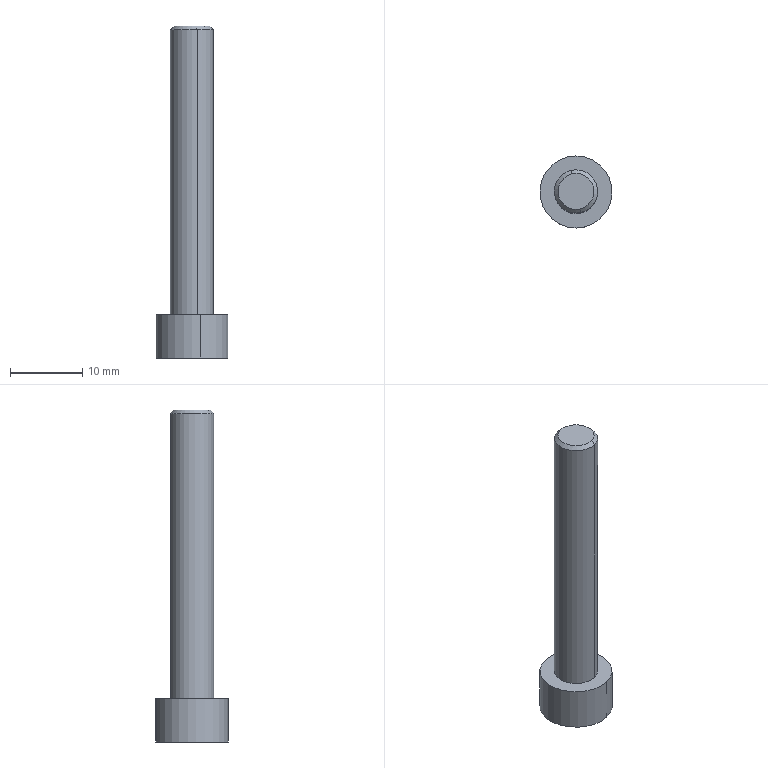Part | SolidWorks | features BaseBody 1 | 1 solid | 16 faces | box 10 x 10 x 46 mm | volume 1535 mm3 | plane 10 | cylinder 4 | cone 2 | commonest cylinder face diameters 6 x2 10 x2
STEP:
#1=CARTESIAN_POINT('',(-84.613,-20.243,-207.85));
#2=VERTEX_POINT('',#1);
#3=CARTESIAN_POINT('',(-87.045,-10.543,-207.85));
#4=VERTEX_POINT('',#3);
#5=CARTESIAN_POINT('',(-85.829,-15.393,-207.85));
#6=DIRECTION('',(0.,0.,1.));
#7=DIRECTION('',(0.2432,-0.97,0.));
#8=AXIS2_PLACEMENT_3D('',#5,#6,#7);
#9=CIRCLE('',#8,5.);
#10=EDGE_CURVE('',#2,#4,#9,.T.);
#11=ORIENTED_EDGE('',*,*,#10,.F.);
#12=CARTESIAN_POINT('',(-84.613,-20.243,-213.85));
#13=VERTEX_POINT('',#12);
#14=CARTESIAN_POINT('',(-84.613,-20.243,-207.85));
#15=DIRECTION('',(0.,0.,-1.));
#16=VECTOR('',#15,1000.);
#17=LINE('',#14,#16);
#18=EDGE_CURVE('',#2,#13,#17,.T.);
#19=ORIENTED_EDGE('',*,*,#18,.T.);
#20=CARTESIAN_POINT('',(-87.045,-10.543,-213.85));
#21=VERTEX_POINT('',#20);
#22=CARTESIAN_POINT('',(-85.829,-15.393,-213.85));
#23=DIRECTION('',(0.,0.,1.));
#24=DIRECTION('',(0.2432,-0.97,0.));
#25=AXIS2_PLACEMENT_3D('',#22,#23,#24);
#26=CIRCLE('',#25,5.);
#27=EDGE_CURVE('',#13,#21,#26,.T.);
#28=ORIENTED_EDGE('',*,*,#27,.T.);
#29=CARTESIAN_POINT('',(-87.045,-10.543,-207.85));
#30=DIRECTION('',(0.,0.,-1.));
#31=VECTOR('',#30,1000.);
#32=LINE('',#29,#31);
#33=EDGE_CURVE('',#4,#21,#32,.T.);
#34=ORIENTED_EDGE('',*,*,#33,.F.);
#35=EDGE_LOOP('',(#11,#19,#28,#34));
#36=FACE_OUTER_BOUND('',#35,.T.);
#37=CARTESIAN_POINT('',(-85.829,-15.393,-207.85));
#38=DIRECTION('',(0.,0.,-1.));
#39=DIRECTION('',(-0.2432,0.97,0.));
#40=AXIS2_PLACEMENT_3D('',#37,#38,#39);
#41=CYLINDRICAL_SURFACE('',#40,5.);
#42=ADVANCED_FACE('',(#36),#41,.T.);
#43=CARTESIAN_POINT('',(-86.559,-12.483,-168.35));
#44=VERTEX_POINT('',#43);
#45=CARTESIAN_POINT('',(-85.1,-18.303,-168.35));
#46=VERTEX_POINT('',#45);
#47=CARTESIAN_POINT('',(-85.829,-15.393,-168.35));
#48=DIRECTION('',(0.,0.,-1.));
#49=DIRECTION('',(0.2432,-0.97,0.));
#50=AXIS2_PLACEMENT_3D('',#47,#48,#49);
#51=CIRCLE('',#50,3.);
#52=EDGE_CURVE('',#44,#46,#51,.T.);
#53=ORIENTED_EDGE('',*,*,#52,.T.);
#54=CARTESIAN_POINT('',(-85.1,-18.303,-207.85));
#55=VERTEX_POINT('',#54);
#56=CARTESIAN_POINT('',(-85.1,-18.303,-167.85));
#57=DIRECTION('',(0.,0.,-1.));
#58=VECTOR('',#57,1000.);
#59=LINE('',#56,#58);
#60=EDGE_CURVE('',#46,#55,#59,.T.);
#61=ORIENTED_EDGE('',*,*,#60,.T.);
#62=CARTESIAN_POINT('',(-86.559,-12.483,-207.85));
#63=VERTEX_POINT('',#62);
#64=CARTESIAN_POINT('',(-85.829,-15.393,-207.85));
#65=DIRECTION('',(0.,0.,1.));
#66=DIRECTION('',(0.2432,-0.97,0.));
#67=AXIS2_PLACEMENT_3D('',#64,#65,#66);
#68=CIRCLE('',#67,3.);
#69=EDGE_CURVE('',#55,#63,#68,.T.);
#70=ORIENTED_EDGE('',*,*,#69,.T.);
#71=CARTESIAN_POINT('',(-86.559,-12.483,-167.85));
#72=DIRECTION('',(0.,0.,-1.));
#73=VECTOR('',#72,1000.);
#74=LINE('',#71,#73);
#75=EDGE_CURVE('',#44,#63,#74,.T.);
#76=ORIENTED_EDGE('',*,*,#75,.F.);
#77=EDGE_LOOP('',(#53,#61,#70,#76));
#78=FACE_OUTER_BOUND('',#77,.T.);
#79=CARTESIAN_POINT('',(-85.829,-15.393,-167.85));
#80=DIRECTION('',(0.,0.,-1.));
#81=DIRECTION('',(-0.2432,0.97,0.));
#82=AXIS2_PLACEMENT_3D('',#79,#80,#81);
#83=CYLINDRICAL_SURFACE('',#82,3.);
#84=ADVANCED_FACE('',(#78),#83,.T.);
#85=CARTESIAN_POINT('',(-85.221,-17.818,-167.85));
#86=VERTEX_POINT('',#85);
#87=CARTESIAN_POINT('',(-86.437,-12.968,-167.85));
#88=VERTEX_POINT('',#87);
#89=CARTESIAN_POINT('',(-85.829,-15.393,-167.85));
#90=DIRECTION('',(0.,0.,1.));
#91=DIRECTION('',(0.2432,-0.97,0.));
#92=AXIS2_PLACEMENT_3D('',#89,#90,#91);
#93=CIRCLE('',#92,2.5);
#94=EDGE_CURVE('',#86,#88,#93,.T.);
#95=ORIENTED_EDGE('',*,*,#94,.F.);
#96=CARTESIAN_POINT('',(-85.221,-17.818,-167.85));
#97=DIRECTION('',(0.1719,-0.6859,-0.7071));
#98=VECTOR('',#97,1000.);
#99=LINE('',#96,#98);
#100=EDGE_CURVE('',#86,#46,#99,.T.);
#101=ORIENTED_EDGE('',*,*,#100,.T.);
#102=ORIENTED_EDGE('',*,*,#52,.F.);
#103=CARTESIAN_POINT('',(-86.437,-12.968,-167.85));
#104=DIRECTION('',(-0.1719,0.6859,-0.7071));
#105=VECTOR('',#104,1000.);
#106=LINE('',#103,#105);
#107=EDGE_CURVE('',#88,#44,#106,.T.);
#108=ORIENTED_EDGE('',*,*,#107,.F.);
#109=EDGE_LOOP('',(#95,#101,#102,#108));
#110=FACE_OUTER_BOUND('',#109,.T.);
#111=CARTESIAN_POINT('',(-85.829,-15.393,-167.85));
#112=DIRECTION('',(0.,0.,-1.));
#113=DIRECTION('',(-0.2432,0.97,0.));
#114=AXIS2_PLACEMENT_3D('',#111,#112,#113);
#115=CONICAL_SURFACE('',#114,2.5,0.7854);
#116=ADVANCED_FACE('',(#110),#115,.T.);
#117=ORIENTED_EDGE('',*,*,#100,.F.);
#118=CARTESIAN_POINT('',(-85.829,-15.393,-167.85));
#119=DIRECTION('',(0.,0.,1.));
#120=DIRECTION('',(0.2432,-0.97,0.));
#121=AXIS2_PLACEMENT_3D('',#118,#119,#120);
#122=CIRCLE('',#121,2.5);
#123=EDGE_CURVE('',#88,#86,#122,.T.);
#124=ORIENTED_EDGE('',*,*,#123,.F.);
#125=ORIENTED_EDGE('',*,*,#107,.T.);
#126=CARTESIAN_POINT('',(-85.829,-15.393,-168.35));
#127=DIRECTION('',(0.,0.,-1.));
#128=DIRECTION('',(0.2432,-0.97,0.));
#129=AXIS2_PLACEMENT_3D('',#126,#127,#128);
#130=CIRCLE('',#129,3.);
#131=EDGE_CURVE('',#46,#44,#130,.T.);
#132=ORIENTED_EDGE('',*,*,#131,.F.);
#133=EDGE_LOOP('',(#117,#124,#125,#132));
#134=FACE_OUTER_BOUND('',#133,.T.);
#135=CARTESIAN_POINT('',(-85.829,-15.393,-167.85));
#136=DIRECTION('',(0.,0.,-1.));
#137=DIRECTION('',(-0.2432,0.97,0.));
#138=AXIS2_PLACEMENT_3D('',#135,#136,#137);
#139=CONICAL_SURFACE('',#138,2.5,0.7854);
#140=ADVANCED_FACE('',(#134),#139,.T.);
#141=CARTESIAN_POINT('',(-83.029,-14.691,-210.85));
#142=VERTEX_POINT('',#141);
#143=CARTESIAN_POINT('',(-83.821,-17.467,-210.85));
#144=VERTEX_POINT('',#143);
#145=CARTESIAN_POINT('',(-83.029,-14.691,-210.85));
#146=DIRECTION('',(-0.2744,-0.9616,0.));
#147=VECTOR('',#146,1000.);
#148=LINE('',#145,#147);
#149=EDGE_CURVE('',#142,#144,#148,.T.);
#150=ORIENTED_EDGE('',*,*,#149,.T.);
#151=CARTESIAN_POINT('',(-86.621,-18.169,-210.85));
#152=VERTEX_POINT('',#151);
#153=CARTESIAN_POINT('',(-83.821,-17.467,-210.85));
#154=DIRECTION('',(-0.97,-0.2432,0.));
#155=VECTOR('',#154,1000.);
#156=LINE('',#153,#155);
#157=EDGE_CURVE('',#144,#152,#156,.T.);
#158=ORIENTED_EDGE('',*,*,#157,.T.);
#159=CARTESIAN_POINT('',(-88.629,-16.095,-210.85));
#160=VERTEX_POINT('',#159);
#161=CARTESIAN_POINT('',(-88.629,-16.095,-210.85));
#162=DIRECTION('',(-0.6956,0.7184,0.));
#163=VECTOR('',#162,1000.);
#164=LINE('',#161,#163);
#165=EDGE_CURVE('',#152,#160,#164,.T.);
#166=ORIENTED_EDGE('',*,*,#165,.T.);
#167=CARTESIAN_POINT('',(-87.837,-13.319,-210.85));
#168=VERTEX_POINT('',#167);
#169=CARTESIAN_POINT('',(-88.629,-16.095,-210.85));
#170=DIRECTION('',(0.2744,0.9616,0.));
#171=VECTOR('',#170,1000.);
#172=LINE('',#169,#171);
#173=EDGE_CURVE('',#160,#168,#172,.T.);
#174=ORIENTED_EDGE('',*,*,#173,.T.);
#175=CARTESIAN_POINT('',(-85.037,-12.617,-210.85));
#176=VERTEX_POINT('',#175);
#177=CARTESIAN_POINT('',(-85.037,-12.617,-210.85));
#178=DIRECTION('',(0.97,0.2432,0.));
#179=VECTOR('',#178,1000.);
#180=LINE('',#177,#179);
#181=EDGE_CURVE('',#168,#176,#180,.T.);
#182=ORIENTED_EDGE('',*,*,#181,.T.);
#183=CARTESIAN_POINT('',(-83.029,-14.691,-210.85));
#184=DIRECTION('',(0.6956,-0.7184,0.));
#185=VECTOR('',#184,1000.);
#186=LINE('',#183,#185);
#187=EDGE_CURVE('',#176,#142,#186,.T.);
#188=ORIENTED_EDGE('',*,*,#187,.T.);
#189=EDGE_LOOP('',(#150,#158,#166,#174,#182,#188));
#190=FACE_OUTER_BOUND('',#189,.T.);
#191=CARTESIAN_POINT('',(-84.613,-20.243,-210.85));
#192=DIRECTION('',(0.,0.,1.));
#193=DIRECTION('',(1.,0.,0.));
#194=AXIS2_PLACEMENT_3D('',#191,#192,#193);
#195=PLANE('',#194);
#196=ADVANCED_FACE('',(#190),#195,.F.);
#197=CARTESIAN_POINT('',(-83.821,-17.467,-213.85));
#198=VERTEX_POINT('',#197);
#199=CARTESIAN_POINT('',(-86.621,-18.169,-213.85));
#200=VERTEX_POINT('',#199);
#201=CARTESIAN_POINT('',(-83.821,-17.467,-213.85));
#202=DIRECTION('',(-0.97,-0.2432,0.));
#203=VECTOR('',#202,1000.);
#204=LINE('',#201,#203);
#205=EDGE_CURVE('',#198,#200,#204,.T.);
#206=ORIENTED_EDGE('',*,*,#205,.T.);
#207=CARTESIAN_POINT('',(-86.621,-18.169,-210.85));
#208=DIRECTION('',(0.,0.,-1.));
#209=VECTOR('',#208,1000.);
#210=LINE('',#207,#209);
#211=EDGE_CURVE('',#152,#200,#210,.T.);
#212=ORIENTED_EDGE('',*,*,#211,.F.);
#213=ORIENTED_EDGE('',*,*,#157,.F.);
#214=CARTESIAN_POINT('',(-83.821,-17.467,-210.85));
#215=DIRECTION('',(0.,0.,-1.));
#216=VECTOR('',#215,1000.);
#217=LINE('',#214,#216);
#218=EDGE_CURVE('',#144,#198,#217,.T.);
#219=ORIENTED_EDGE('',*,*,#218,.T.);
#220=EDGE_LOOP('',(#206,#212,#213,#219));
#221=FACE_OUTER_BOUND('',#220,.T.);
#222=CARTESIAN_POINT('',(-83.821,-17.467,-210.85));
#223=DIRECTION('',(0.2432,-0.97,0.));
#224=DIRECTION('',(0.,0.,-1.));
#225=AXIS2_PLACEMENT_3D('',#222,#223,#224);
#226=PLANE('',#225);
#227=ADVANCED_FACE('',(#221),#226,.F.);
#228=CARTESIAN_POINT('',(-88.629,-16.095,-213.85));
#229=VERTEX_POINT('',#228);
#230=CARTESIAN_POINT('',(-88.629,-16.095,-213.85));
#231=DIRECTION('',(-0.6956,0.7184,0.));
#232=VECTOR('',#231,1000.);
#233=LINE('',#230,#232);
#234=EDGE_CURVE('',#200,#229,#233,.T.);
#235=ORIENTED_EDGE('',*,*,#234,.T.);
#236=CARTESIAN_POINT('',(-88.629,-16.095,-210.85));
#237=DIRECTION('',(0.,0.,-1.));
#238=VECTOR('',#237,1000.);
#239=LINE('',#236,#238);
#240=EDGE_CURVE('',#160,#229,#239,.T.);
#241=ORIENTED_EDGE('',*,*,#240,.F.);
#242=ORIENTED_EDGE('',*,*,#165,.F.);
#243=ORIENTED_EDGE('',*,*,#211,.T.);
#244=EDGE_LOOP('',(#235,#241,#242,#243));
#245=FACE_OUTER_BOUND('',#244,.T.);
#246=CARTESIAN_POINT('',(-88.629,-16.095,-210.85));
#247=DIRECTION('',(-0.7184,-0.6956,0.));
#248=DIRECTION('',(-0.6956,0.7184,0.));
#249=AXIS2_PLACEMENT_3D('',#246,#247,#248);
#250=PLANE('',#249);
#251=ADVANCED_FACE('',(#245),#250,.F.);
#252=CARTESIAN_POINT('',(-87.837,-13.319,-213.85));
#253=VERTEX_POINT('',#252);
#254=CARTESIAN_POINT('',(-88.629,-16.095,-213.85));
#255=DIRECTION('',(0.2744,0.9616,0.));
#256=VECTOR('',#255,1000.);
#257=LINE('',#254,#256);
#258=EDGE_CURVE('',#229,#253,#257,.T.);
#259=ORIENTED_EDGE('',*,*,#258,.T.);
#260=CARTESIAN_POINT('',(-87.837,-13.319,-210.85));
#261=DIRECTION('',(0.,0.,-1.));
#262=VECTOR('',#261,1000.);
#263=LINE('',#260,#262);
#264=EDGE_CURVE('',#168,#253,#263,.T.);
#265=ORIENTED_EDGE('',*,*,#264,.F.);
#266=ORIENTED_EDGE('',*,*,#173,.F.);
#267=ORIENTED_EDGE('',*,*,#240,.T.);
#268=EDGE_LOOP('',(#259,#265,#266,#267));
#269=FACE_OUTER_BOUND('',#268,.T.);
#270=CARTESIAN_POINT('',(-88.629,-16.095,-210.85));
#271=DIRECTION('',(-0.9616,0.2744,0.));
#272=DIRECTION('',(0.,0.,1.));
#273=AXIS2_PLACEMENT_3D('',#270,#271,#272);
#274=PLANE('',#273);
#275=ADVANCED_FACE('',(#269),#274,.F.);
#276=CARTESIAN_POINT('',(-85.037,-12.617,-213.85));
#277=VERTEX_POINT('',#276);
#278=CARTESIAN_POINT('',(-85.037,-12.617,-213.85));
#279=DIRECTION('',(0.97,0.2432,0.));
#280=VECTOR('',#279,1000.);
#281=LINE('',#278,#280);
#282=EDGE_CURVE('',#253,#277,#281,.T.);
#283=ORIENTED_EDGE('',*,*,#282,.T.);
#284=CARTESIAN_POINT('',(-85.037,-12.617,-210.85));
#285=DIRECTION('',(0.,0.,-1.));
#286=VECTOR('',#285,1000.);
#287=LINE('',#284,#286);
#288=EDGE_CURVE('',#176,#277,#287,.T.);
#289=ORIENTED_EDGE('',*,*,#288,.F.);
#290=ORIENTED_EDGE('',*,*,#181,.F.);
#291=ORIENTED_EDGE('',*,*,#264,.T.);
#292=EDGE_LOOP('',(#283,#289,#290,#291));
#293=FACE_OUTER_BOUND('',#292,.T.);
#294=CARTESIAN_POINT('',(-85.037,-12.617,-210.85));
#295=DIRECTION('',(-0.2432,0.97,0.));
#296=DIRECTION('',(0.,0.,1.));
#297=AXIS2_PLACEMENT_3D('',#294,#295,#296);
#298=PLANE('',#297);
#299=ADVANCED_FACE('',(#293),#298,.F.);
#300=CARTESIAN_POINT('',(-83.029,-14.691,-213.85));
#301=VERTEX_POINT('',#300);
#302=CARTESIAN_POINT('',(-83.029,-14.691,-213.85));
#303=DIRECTION('',(0.6956,-0.7184,0.));
#304=VECTOR('',#303,1000.);
#305=LINE('',#302,#304);
#306=EDGE_CURVE('',#277,#301,#305,.T.);
#307=ORIENTED_EDGE('',*,*,#306,.T.);
#308=CARTESIAN_POINT('',(-83.029,-14.691,-210.85));
#309=DIRECTION('',(0.,0.,-1.));
#310=VECTOR('',#309,1000.);
#311=LINE('',#308,#310);
#312=EDGE_CURVE('',#142,#301,#311,.T.);
#313=ORIENTED_EDGE('',*,*,#312,.F.);
#314=ORIENTED_EDGE('',*,*,#187,.F.);
#315=ORIENTED_EDGE('',*,*,#288,.T.);
#316=EDGE_LOOP('',(#307,#313,#314,#315));
#317=FACE_OUTER_BOUND('',#316,.T.);
#318=CARTESIAN_POINT('',(-83.029,-14.691,-210.85));
#319=DIRECTION('',(0.7184,0.6956,0.));
#320=DIRECTION('',(0.,0.,-1.));
#321=AXIS2_PLACEMENT_3D('',#318,#319,#320);
#322=PLANE('',#321);
#323=ADVANCED_FACE('',(#317),#322,.F.);
#324=CARTESIAN_POINT('',(-83.029,-14.691,-213.85));
#325=DIRECTION('',(-0.2744,-0.9616,0.));
#326=VECTOR('',#325,1000.);
#327=LINE('',#324,#326);
#328=EDGE_CURVE('',#301,#198,#327,.T.);
#329=ORIENTED_EDGE('',*,*,#328,.T.);
#330=ORIENTED_EDGE('',*,*,#218,.F.);
#331=ORIENTED_EDGE('',*,*,#149,.F.);
#332=ORIENTED_EDGE('',*,*,#312,.T.);
#333=EDGE_LOOP('',(#329,#330,#331,#332));
#334=FACE_OUTER_BOUND('',#333,.T.);
#335=CARTESIAN_POINT('',(-83.029,-14.691,-210.85));
#336=DIRECTION('',(0.9616,-0.2744,0.));
#337=DIRECTION('',(0.,0.,-1.));
#338=AXIS2_PLACEMENT_3D('',#335,#336,#337);
#339=PLANE('',#338);
#340=ADVANCED_FACE('',(#334),#339,.F.);
#341=ORIENTED_EDGE('',*,*,#123,.T.);
#342=ORIENTED_EDGE('',*,*,#94,.T.);
#343=EDGE_LOOP('',(#341,#342));
#344=FACE_OUTER_BOUND('',#343,.T.);
#345=CARTESIAN_POINT('',(-85.829,-15.393,-167.85));
#346=DIRECTION('',(0.,0.,1.));
#347=DIRECTION('',(1.,0.,0.));
#348=AXIS2_PLACEMENT_3D('',#345,#346,#347);
#349=PLANE('',#348);
#350=ADVANCED_FACE('',(#344),#349,.T.);
#351=ORIENTED_EDGE('',*,*,#60,.F.);
#352=ORIENTED_EDGE('',*,*,#131,.T.);
#353=ORIENTED_EDGE('',*,*,#75,.T.);
#354=CARTESIAN_POINT('',(-85.829,-15.393,-207.85));
#355=DIRECTION('',(0.,0.,1.));
#356=DIRECTION('',(0.2432,-0.97,0.));
#357=AXIS2_PLACEMENT_3D('',#354,#355,#356);
#358=CIRCLE('',#357,3.);
#359=EDGE_CURVE('',#63,#55,#358,.T.);
#360=ORIENTED_EDGE('',*,*,#359,.T.);
#361=EDGE_LOOP('',(#351,#352,#353,#360));
#362=FACE_OUTER_BOUND('',#361,.T.);
#363=CARTESIAN_POINT('',(-85.829,-15.393,-167.85));
#364=DIRECTION('',(0.,0.,-1.));
#365=DIRECTION('',(-0.2432,0.97,0.));
#366=AXIS2_PLACEMENT_3D('',#363,#364,#365);
#367=CYLINDRICAL_SURFACE('',#366,3.);
#368=ADVANCED_FACE('',(#362),#367,.T.);
#369=CARTESIAN_POINT('',(-85.829,-15.393,-213.85));
#370=DIRECTION('',(0.,0.,1.));
#371=DIRECTION('',(0.2432,-0.97,0.));
#372=AXIS2_PLACEMENT_3D('',#369,#370,#371);
#373=CIRCLE('',#372,5.);
#374=EDGE_CURVE('',#21,#13,#373,.T.);
#375=ORIENTED_EDGE('',*,*,#374,.F.);
#376=ORIENTED_EDGE('',*,*,#27,.F.);
#377=EDGE_LOOP('',(#375,#376));
#378=FACE_OUTER_BOUND('',#377,.T.);
#379=ORIENTED_EDGE('',*,*,#205,.F.);
#380=ORIENTED_EDGE('',*,*,#328,.F.);
#381=ORIENTED_EDGE('',*,*,#306,.F.);
#382=ORIENTED_EDGE('',*,*,#282,.F.);
#383=ORIENTED_EDGE('',*,*,#258,.F.);
#384=ORIENTED_EDGE('',*,*,#234,.F.);
#385=EDGE_LOOP('',(#379,#380,#381,#382,#383,#384));
#386=FACE_BOUND('',#385,.T.);
#387=CARTESIAN_POINT('',(-85.829,-15.393,-213.85));
#388=DIRECTION('',(0.,0.,1.));
#389=DIRECTION('',(1.,0.,0.));
#390=AXIS2_PLACEMENT_3D('',#387,#388,#389);
#391=PLANE('',#390);
#392=ADVANCED_FACE('',(#378,#386),#391,.F.);
#393=ORIENTED_EDGE('',*,*,#18,.F.);
#394=CARTESIAN_POINT('',(-85.829,-15.393,-207.85));
#395=DIRECTION('',(0.,0.,1.));
#396=DIRECTION('',(0.2432,-0.97,0.));
#397=AXIS2_PLACEMENT_3D('',#394,#395,#396);
#398=CIRCLE('',#397,5.);
#399=EDGE_CURVE('',#4,#2,#398,.T.);
#400=ORIENTED_EDGE('',*,*,#399,.F.);
#401=ORIENTED_EDGE('',*,*,#33,.T.);
#402=ORIENTED_EDGE('',*,*,#374,.T.);
#403=EDGE_LOOP('',(#393,#400,#401,#402));
#404=FACE_OUTER_BOUND('',#403,.T.);
#405=CARTESIAN_POINT('',(-85.829,-15.393,-207.85));
#406=DIRECTION('',(0.,0.,-1.));
#407=DIRECTION('',(-0.2432,0.97,0.));
#408=AXIS2_PLACEMENT_3D('',#405,#406,#407);
#409=CYLINDRICAL_SURFACE('',#408,5.);
#410=ADVANCED_FACE('',(#404),#409,.T.);
#411=ORIENTED_EDGE('',*,*,#359,.F.);
#412=ORIENTED_EDGE('',*,*,#69,.F.);
#413=EDGE_LOOP('',(#411,#412));
#414=FACE_BOUND('',#413,.T.);
#415=ORIENTED_EDGE('',*,*,#399,.T.);
#416=ORIENTED_EDGE('',*,*,#10,.T.);
#417=EDGE_LOOP('',(#415,#416));
#418=FACE_OUTER_BOUND('',#417,.T.);
#419=CARTESIAN_POINT('',(-85.829,-15.393,-207.85));
#420=DIRECTION('',(0.,0.,1.));
#421=DIRECTION('',(1.,0.,0.));
#422=AXIS2_PLACEMENT_3D('',#419,#420,#421);
#423=PLANE('',#422);
#424=ADVANCED_FACE('',(#414,#418),#423,.T.);
#425=CLOSED_SHELL('',(#42,#84,#116,#140,#196,#227,#251,#275,#299,#323,#340,#350,#368,#392,#410,#424));
#426=MANIFOLD_SOLID_BREP('',#425);
#427=CARTESIAN_POINT('',(0.,0.,0.));
#428=DIRECTION('',(0.,0.,1.));
#429=DIRECTION('',(1.,0.,0.));
#430=AXIS2_PLACEMENT_3D('',#427,#428,#429);
#431=(LENGTH_UNIT()NAMED_UNIT(*)SI_UNIT(.MILLI.,.METRE.));
#432=UNCERTAINTY_MEASURE_WITH_UNIT(LENGTH_MEASURE(0.00001),#431,'','');
#433=(NAMED_UNIT(*)PLANE_ANGLE_UNIT()SI_UNIT($,.RADIAN.));
#434=(NAMED_UNIT(*)SI_UNIT($,.STERADIAN.)SOLID_ANGLE_UNIT());
#435=(GEOMETRIC_REPRESENTATION_CONTEXT(3)GLOBAL_UNCERTAINTY_ASSIGNED_CONTEXT((#432))GLOBAL_UNIT_ASSIGNED_CONTEXT((#431,#433,#434))REPRESENTATION_CONTEXT('',''));
#436=ADVANCED_BREP_SHAPE_REPRESENTATION('',(#426,#430),#435);